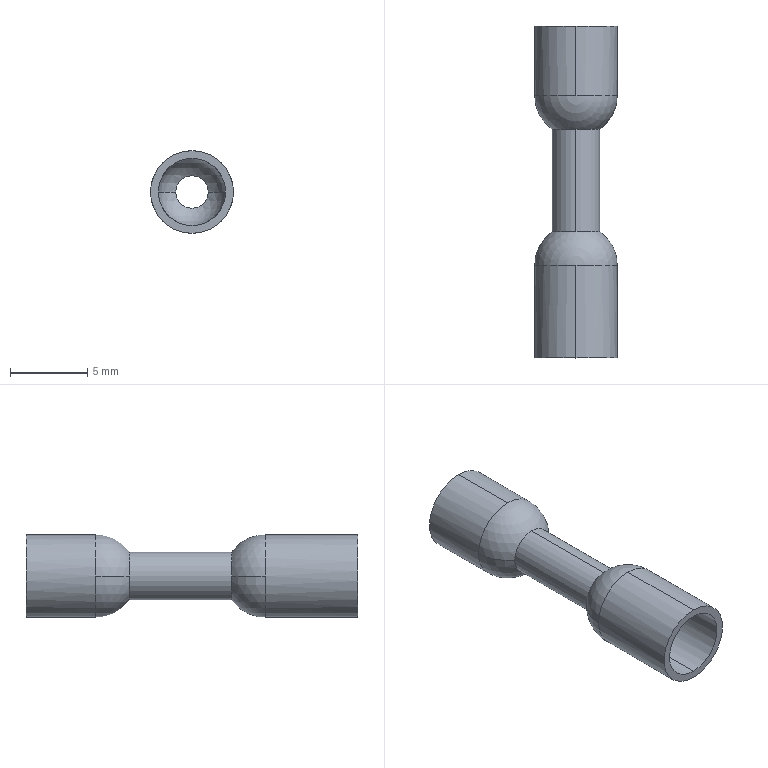Part | SolidWorks | features RevolutionThin 1 | 1 solid | 22 faces | box 5.36 x 21.494 x 5.36 mm | volume 139.623 mm3 | cylinder 12 | sphere 8 | plane 2 | commonest cylinder face diameters 4.36 x4 5.36 x4 2.1 x2 3.1 x2
STEP:
#1=CARTESIAN_POINT('',(0.,6.,2.68));
#2=VERTEX_POINT('',#1);
#3=CARTESIAN_POINT('',(2.68,6.,0.));
#4=VERTEX_POINT('',#3);
#5=CARTESIAN_POINT('',(0.,6.,0.));
#6=DIRECTION('',(0.,1.,0.));
#7=DIRECTION('',(0.,0.,1.));
#8=AXIS2_PLACEMENT_3D('',#5,#6,#7);
#9=CIRCLE('',#8,2.68);
#10=EDGE_CURVE('',#2,#4,#9,.T.);
#11=ORIENTED_EDGE('',*,*,#10,.T.);
#12=CARTESIAN_POINT('',(1.55,8.186,0.));
#13=VERTEX_POINT('',#12);
#14=CARTESIAN_POINT('',(0.,6.,0.));
#15=DIRECTION('',(0.,0.,1.));
#16=DIRECTION('',(1.,0.,0.));
#17=AXIS2_PLACEMENT_3D('',#14,#15,#16);
#18=CIRCLE('',#17,2.68);
#19=EDGE_CURVE('',#4,#13,#18,.T.);
#20=ORIENTED_EDGE('',*,*,#19,.T.);
#21=CARTESIAN_POINT('',(0.,8.186,1.55));
#22=VERTEX_POINT('',#21);
#23=CARTESIAN_POINT('',(0.,8.186,0.));
#24=DIRECTION('',(0.,1.,0.));
#25=DIRECTION('',(0.,0.,1.));
#26=AXIS2_PLACEMENT_3D('',#23,#24,#25);
#27=CIRCLE('',#26,1.55);
#28=EDGE_CURVE('',#22,#13,#27,.T.);
#29=ORIENTED_EDGE('',*,*,#28,.F.);
#30=CARTESIAN_POINT('',(-1.55,8.186,0.));
#31=VERTEX_POINT('',#30);
#32=CARTESIAN_POINT('',(0.,8.186,0.));
#33=DIRECTION('',(0.,1.,0.));
#34=DIRECTION('',(0.,0.,1.));
#35=AXIS2_PLACEMENT_3D('',#32,#33,#34);
#36=CIRCLE('',#35,1.55);
#37=EDGE_CURVE('',#31,#22,#36,.T.);
#38=ORIENTED_EDGE('',*,*,#37,.F.);
#39=CARTESIAN_POINT('',(-2.68,6.,0.));
#40=VERTEX_POINT('',#39);
#41=CARTESIAN_POINT('',(0.,6.,0.));
#42=DIRECTION('',(0.,0.,-1.));
#43=DIRECTION('',(-1.,0.,0.));
#44=AXIS2_PLACEMENT_3D('',#41,#42,#43);
#45=CIRCLE('',#44,2.68);
#46=EDGE_CURVE('',#40,#31,#45,.T.);
#47=ORIENTED_EDGE('',*,*,#46,.F.);
#48=CARTESIAN_POINT('',(0.,6.,0.));
#49=DIRECTION('',(0.,1.,0.));
#50=DIRECTION('',(0.,0.,1.));
#51=AXIS2_PLACEMENT_3D('',#48,#49,#50);
#52=CIRCLE('',#51,2.68);
#53=EDGE_CURVE('',#40,#2,#52,.T.);
#54=ORIENTED_EDGE('',*,*,#53,.T.);
#55=EDGE_LOOP('',(#11,#20,#29,#38,#47,#54));
#56=FACE_OUTER_BOUND('',#55,.T.);
#57=CARTESIAN_POINT('',(0.,6.,0.));
#58=DIRECTION('',(0.,0.,1.));
#59=DIRECTION('',(-1.,0.,0.));
#60=AXIS2_PLACEMENT_3D('',#57,#58,#59);
#61=SPHERICAL_SURFACE('',#60,2.68);
#62=ADVANCED_FACE('',(#56),#61,.T.);
#63=ORIENTED_EDGE('',*,*,#28,.T.);
#64=CARTESIAN_POINT('',(0.,8.186,-1.55));
#65=VERTEX_POINT('',#64);
#66=CARTESIAN_POINT('',(0.,8.186,0.));
#67=DIRECTION('',(0.,1.,0.));
#68=DIRECTION('',(0.,0.,1.));
#69=AXIS2_PLACEMENT_3D('',#66,#67,#68);
#70=CIRCLE('',#69,1.55);
#71=EDGE_CURVE('',#13,#65,#70,.T.);
#72=ORIENTED_EDGE('',*,*,#71,.T.);
#73=CARTESIAN_POINT('',(0.,14.808,-1.55));
#74=VERTEX_POINT('',#73);
#75=CARTESIAN_POINT('',(0.,24.172,-1.55));
#76=DIRECTION('',(0.,1.,0.));
#77=VECTOR('',#76,1000.);
#78=LINE('',#75,#77);
#79=EDGE_CURVE('',#65,#74,#78,.T.);
#80=ORIENTED_EDGE('',*,*,#79,.T.);
#81=CARTESIAN_POINT('',(1.55,14.808,0.));
#82=VERTEX_POINT('',#81);
#83=CARTESIAN_POINT('',(0.,14.808,0.));
#84=DIRECTION('',(0.,1.,0.));
#85=DIRECTION('',(0.,0.,1.));
#86=AXIS2_PLACEMENT_3D('',#83,#84,#85);
#87=CIRCLE('',#86,1.55);
#88=EDGE_CURVE('',#82,#74,#87,.T.);
#89=ORIENTED_EDGE('',*,*,#88,.F.);
#90=CARTESIAN_POINT('',(0.,14.808,1.55));
#91=VERTEX_POINT('',#90);
#92=CARTESIAN_POINT('',(0.,14.808,0.));
#93=DIRECTION('',(0.,1.,0.));
#94=DIRECTION('',(0.,0.,1.));
#95=AXIS2_PLACEMENT_3D('',#92,#93,#94);
#96=CIRCLE('',#95,1.55);
#97=EDGE_CURVE('',#91,#82,#96,.T.);
#98=ORIENTED_EDGE('',*,*,#97,.F.);
#99=CARTESIAN_POINT('',(0.,24.172,1.55));
#100=DIRECTION('',(0.,1.,0.));
#101=VECTOR('',#100,1000.);
#102=LINE('',#99,#101);
#103=EDGE_CURVE('',#22,#91,#102,.T.);
#104=ORIENTED_EDGE('',*,*,#103,.F.);
#105=EDGE_LOOP('',(#63,#72,#80,#89,#98,#104));
#106=FACE_OUTER_BOUND('',#105,.T.);
#107=CARTESIAN_POINT('',(0.,24.172,0.));
#108=DIRECTION('',(0.,1.,0.));
#109=DIRECTION('',(0.,0.,1.));
#110=AXIS2_PLACEMENT_3D('',#107,#108,#109);
#111=CYLINDRICAL_SURFACE('',#110,1.55);
#112=ADVANCED_FACE('',(#106),#111,.T.);
#113=CARTESIAN_POINT('',(-1.55,14.808,0.));
#114=VERTEX_POINT('',#113);
#115=CARTESIAN_POINT('',(0.,14.808,0.));
#116=DIRECTION('',(0.,1.,0.));
#117=DIRECTION('',(0.,0.,1.));
#118=AXIS2_PLACEMENT_3D('',#115,#116,#117);
#119=CIRCLE('',#118,1.55);
#120=EDGE_CURVE('',#114,#91,#119,.T.);
#121=ORIENTED_EDGE('',*,*,#120,.T.);
#122=ORIENTED_EDGE('',*,*,#97,.T.);
#123=CARTESIAN_POINT('',(2.68,16.994,0.));
#124=VERTEX_POINT('',#123);
#125=CARTESIAN_POINT('',(0.,16.994,0.));
#126=DIRECTION('',(0.,0.,1.));
#127=DIRECTION('',(1.,0.,0.));
#128=AXIS2_PLACEMENT_3D('',#125,#126,#127);
#129=CIRCLE('',#128,2.68);
#130=EDGE_CURVE('',#82,#124,#129,.T.);
#131=ORIENTED_EDGE('',*,*,#130,.T.);
#132=CARTESIAN_POINT('',(0.,16.994,2.68));
#133=VERTEX_POINT('',#132);
#134=CARTESIAN_POINT('',(0.,16.994,0.));
#135=DIRECTION('',(0.,1.,0.));
#136=DIRECTION('',(0.,0.,1.));
#137=AXIS2_PLACEMENT_3D('',#134,#135,#136);
#138=CIRCLE('',#137,2.68);
#139=EDGE_CURVE('',#133,#124,#138,.T.);
#140=ORIENTED_EDGE('',*,*,#139,.F.);
#141=CARTESIAN_POINT('',(-2.68,16.994,0.));
#142=VERTEX_POINT('',#141);
#143=CARTESIAN_POINT('',(0.,16.994,0.));
#144=DIRECTION('',(0.,1.,0.));
#145=DIRECTION('',(0.,0.,1.));
#146=AXIS2_PLACEMENT_3D('',#143,#144,#145);
#147=CIRCLE('',#146,2.68);
#148=EDGE_CURVE('',#142,#133,#147,.T.);
#149=ORIENTED_EDGE('',*,*,#148,.F.);
#150=CARTESIAN_POINT('',(0.,16.994,0.));
#151=DIRECTION('',(0.,0.,-1.));
#152=DIRECTION('',(-1.,0.,0.));
#153=AXIS2_PLACEMENT_3D('',#150,#151,#152);
#154=CIRCLE('',#153,2.68);
#155=EDGE_CURVE('',#114,#142,#154,.T.);
#156=ORIENTED_EDGE('',*,*,#155,.F.);
#157=EDGE_LOOP('',(#121,#122,#131,#140,#149,#156));
#158=FACE_OUTER_BOUND('',#157,.T.);
#159=CARTESIAN_POINT('',(0.,16.994,0.));
#160=DIRECTION('',(0.,0.,1.));
#161=DIRECTION('',(-1.,0.,0.));
#162=AXIS2_PLACEMENT_3D('',#159,#160,#161);
#163=SPHERICAL_SURFACE('',#162,2.68);
#164=ADVANCED_FACE('',(#158),#163,.T.);
#165=ORIENTED_EDGE('',*,*,#139,.T.);
#166=CARTESIAN_POINT('',(0.,16.994,-2.68));
#167=VERTEX_POINT('',#166);
#168=CARTESIAN_POINT('',(0.,16.994,0.));
#169=DIRECTION('',(0.,1.,0.));
#170=DIRECTION('',(0.,0.,1.));
#171=AXIS2_PLACEMENT_3D('',#168,#169,#170);
#172=CIRCLE('',#171,2.68);
#173=EDGE_CURVE('',#124,#167,#172,.T.);
#174=ORIENTED_EDGE('',*,*,#173,.T.);
#175=CARTESIAN_POINT('',(0.,21.494,-2.68));
#176=VERTEX_POINT('',#175);
#177=CARTESIAN_POINT('',(0.,24.172,-2.68));
#178=DIRECTION('',(0.,1.,0.));
#179=VECTOR('',#178,1000.);
#180=LINE('',#177,#179);
#181=EDGE_CURVE('',#167,#176,#180,.T.);
#182=ORIENTED_EDGE('',*,*,#181,.T.);
#183=CARTESIAN_POINT('',(0.,21.494,2.68));
#184=VERTEX_POINT('',#183);
#185=CARTESIAN_POINT('',(0.,21.494,0.));
#186=DIRECTION('',(0.,1.,0.));
#187=DIRECTION('',(0.,0.,1.));
#188=AXIS2_PLACEMENT_3D('',#185,#186,#187);
#189=CIRCLE('',#188,2.68);
#190=EDGE_CURVE('',#184,#176,#189,.T.);
#191=ORIENTED_EDGE('',*,*,#190,.F.);
#192=CARTESIAN_POINT('',(0.,24.172,2.68));
#193=DIRECTION('',(0.,1.,0.));
#194=VECTOR('',#193,1000.);
#195=LINE('',#192,#194);
#196=EDGE_CURVE('',#133,#184,#195,.T.);
#197=ORIENTED_EDGE('',*,*,#196,.F.);
#198=EDGE_LOOP('',(#165,#174,#182,#191,#197));
#199=FACE_OUTER_BOUND('',#198,.T.);
#200=CARTESIAN_POINT('',(0.,24.172,0.));
#201=DIRECTION('',(0.,1.,0.));
#202=DIRECTION('',(0.,0.,1.));
#203=AXIS2_PLACEMENT_3D('',#200,#201,#202);
#204=CYLINDRICAL_SURFACE('',#203,2.68);
#205=ADVANCED_FACE('',(#199),#204,.T.);
#206=CARTESIAN_POINT('',(0.,16.994,-2.18));
#207=VERTEX_POINT('',#206);
#208=CARTESIAN_POINT('',(-2.18,16.994,0.));
#209=VERTEX_POINT('',#208);
#210=CARTESIAN_POINT('',(0.,16.994,0.));
#211=DIRECTION('',(0.,1.,0.));
#212=DIRECTION('',(0.,0.,1.));
#213=AXIS2_PLACEMENT_3D('',#210,#211,#212);
#214=CIRCLE('',#213,2.18);
#215=EDGE_CURVE('',#207,#209,#214,.T.);
#216=ORIENTED_EDGE('',*,*,#215,.F.);
#217=CARTESIAN_POINT('',(0.,21.494,-2.18));
#218=VERTEX_POINT('',#217);
#219=CARTESIAN_POINT('',(0.,24.172,-2.18));
#220=DIRECTION('',(0.,1.,0.));
#221=VECTOR('',#220,1000.);
#222=LINE('',#219,#221);
#223=EDGE_CURVE('',#207,#218,#222,.T.);
#224=ORIENTED_EDGE('',*,*,#223,.T.);
#225=CARTESIAN_POINT('',(0.,21.494,2.18));
#226=VERTEX_POINT('',#225);
#227=CARTESIAN_POINT('',(0.,21.494,0.));
#228=DIRECTION('',(0.,1.,0.));
#229=DIRECTION('',(0.,0.,1.));
#230=AXIS2_PLACEMENT_3D('',#227,#228,#229);
#231=CIRCLE('',#230,2.18);
#232=EDGE_CURVE('',#218,#226,#231,.T.);
#233=ORIENTED_EDGE('',*,*,#232,.T.);
#234=CARTESIAN_POINT('',(0.,16.994,2.18));
#235=VERTEX_POINT('',#234);
#236=CARTESIAN_POINT('',(0.,24.172,2.18));
#237=DIRECTION('',(0.,1.,0.));
#238=VECTOR('',#237,1000.);
#239=LINE('',#236,#238);
#240=EDGE_CURVE('',#235,#226,#239,.T.);
#241=ORIENTED_EDGE('',*,*,#240,.F.);
#242=CARTESIAN_POINT('',(0.,16.994,0.));
#243=DIRECTION('',(0.,1.,0.));
#244=DIRECTION('',(0.,0.,1.));
#245=AXIS2_PLACEMENT_3D('',#242,#243,#244);
#246=CIRCLE('',#245,2.18);
#247=EDGE_CURVE('',#209,#235,#246,.T.);
#248=ORIENTED_EDGE('',*,*,#247,.F.);
#249=EDGE_LOOP('',(#216,#224,#233,#241,#248));
#250=FACE_OUTER_BOUND('',#249,.T.);
#251=CARTESIAN_POINT('',(0.,24.172,0.));
#252=DIRECTION('',(0.,1.,0.));
#253=DIRECTION('',(0.,0.,1.));
#254=AXIS2_PLACEMENT_3D('',#251,#252,#253);
#255=CYLINDRICAL_SURFACE('',#254,2.18);
#256=ADVANCED_FACE('',(#250),#255,.F.);
#257=CARTESIAN_POINT('',(1.05,15.083,0.));
#258=VERTEX_POINT('',#257);
#259=CARTESIAN_POINT('',(0.,15.083,-1.05));
#260=VERTEX_POINT('',#259);
#261=CARTESIAN_POINT('',(0.,15.083,0.));
#262=DIRECTION('',(0.,1.,0.));
#263=DIRECTION('',(0.,0.,1.));
#264=AXIS2_PLACEMENT_3D('',#261,#262,#263);
#265=CIRCLE('',#264,1.05);
#266=EDGE_CURVE('',#258,#260,#265,.T.);
#267=ORIENTED_EDGE('',*,*,#266,.F.);
#268=CARTESIAN_POINT('',(2.18,16.994,0.));
#269=VERTEX_POINT('',#268);
#270=CARTESIAN_POINT('',(0.,16.994,0.));
#271=DIRECTION('',(0.,0.,1.));
#272=DIRECTION('',(1.,0.,0.));
#273=AXIS2_PLACEMENT_3D('',#270,#271,#272);
#274=CIRCLE('',#273,2.18);
#275=EDGE_CURVE('',#258,#269,#274,.T.);
#276=ORIENTED_EDGE('',*,*,#275,.T.);
#277=CARTESIAN_POINT('',(0.,16.994,0.));
#278=DIRECTION('',(0.,1.,0.));
#279=DIRECTION('',(0.,0.,1.));
#280=AXIS2_PLACEMENT_3D('',#277,#278,#279);
#281=CIRCLE('',#280,2.18);
#282=EDGE_CURVE('',#269,#207,#281,.T.);
#283=ORIENTED_EDGE('',*,*,#282,.T.);
#284=ORIENTED_EDGE('',*,*,#215,.T.);
#285=CARTESIAN_POINT('',(-1.05,15.083,0.));
#286=VERTEX_POINT('',#285);
#287=CARTESIAN_POINT('',(0.,16.994,0.));
#288=DIRECTION('',(0.,0.,-1.));
#289=DIRECTION('',(-1.,0.,0.));
#290=AXIS2_PLACEMENT_3D('',#287,#288,#289);
#291=CIRCLE('',#290,2.18);
#292=EDGE_CURVE('',#286,#209,#291,.T.);
#293=ORIENTED_EDGE('',*,*,#292,.F.);
#294=CARTESIAN_POINT('',(0.,15.083,0.));
#295=DIRECTION('',(0.,1.,0.));
#296=DIRECTION('',(0.,0.,1.));
#297=AXIS2_PLACEMENT_3D('',#294,#295,#296);
#298=CIRCLE('',#297,1.05);
#299=EDGE_CURVE('',#260,#286,#298,.T.);
#300=ORIENTED_EDGE('',*,*,#299,.F.);
#301=EDGE_LOOP('',(#267,#276,#283,#284,#293,#300));
#302=FACE_OUTER_BOUND('',#301,.T.);
#303=CARTESIAN_POINT('',(0.,16.994,0.));
#304=DIRECTION('',(0.,0.,1.));
#305=DIRECTION('',(-1.,0.,0.));
#306=AXIS2_PLACEMENT_3D('',#303,#304,#305);
#307=SPHERICAL_SURFACE('',#306,2.18);
#308=ADVANCED_FACE('',(#302),#307,.F.);
#309=CARTESIAN_POINT('',(0.,7.91,-1.05));
#310=VERTEX_POINT('',#309);
#311=CARTESIAN_POINT('',(-1.05,7.91,0.));
#312=VERTEX_POINT('',#311);
#313=CARTESIAN_POINT('',(0.,7.91,0.));
#314=DIRECTION('',(0.,1.,0.));
#315=DIRECTION('',(0.,0.,1.));
#316=AXIS2_PLACEMENT_3D('',#313,#314,#315);
#317=CIRCLE('',#316,1.05);
#318=EDGE_CURVE('',#310,#312,#317,.T.);
#319=ORIENTED_EDGE('',*,*,#318,.F.);
#320=CARTESIAN_POINT('',(0.,24.172,-1.05));
#321=DIRECTION('',(0.,1.,0.));
#322=VECTOR('',#321,1000.);
#323=LINE('',#320,#322);
#324=EDGE_CURVE('',#310,#260,#323,.T.);
#325=ORIENTED_EDGE('',*,*,#324,.T.);
#326=ORIENTED_EDGE('',*,*,#299,.T.);
#327=CARTESIAN_POINT('',(0.,15.083,1.05));
#328=VERTEX_POINT('',#327);
#329=CARTESIAN_POINT('',(0.,15.083,0.));
#330=DIRECTION('',(0.,1.,0.));
#331=DIRECTION('',(0.,0.,1.));
#332=AXIS2_PLACEMENT_3D('',#329,#330,#331);
#333=CIRCLE('',#332,1.05);
#334=EDGE_CURVE('',#286,#328,#333,.T.);
#335=ORIENTED_EDGE('',*,*,#334,.T.);
#336=CARTESIAN_POINT('',(0.,7.91,1.05));
#337=VERTEX_POINT('',#336);
#338=CARTESIAN_POINT('',(0.,24.172,1.05));
#339=DIRECTION('',(0.,1.,0.));
#340=VECTOR('',#339,1000.);
#341=LINE('',#338,#340);
#342=EDGE_CURVE('',#337,#328,#341,.T.);
#343=ORIENTED_EDGE('',*,*,#342,.F.);
#344=CARTESIAN_POINT('',(0.,7.91,0.));
#345=DIRECTION('',(0.,1.,0.));
#346=DIRECTION('',(0.,0.,1.));
#347=AXIS2_PLACEMENT_3D('',#344,#345,#346);
#348=CIRCLE('',#347,1.05);
#349=EDGE_CURVE('',#312,#337,#348,.T.);
#350=ORIENTED_EDGE('',*,*,#349,.F.);
#351=EDGE_LOOP('',(#319,#325,#326,#335,#343,#350));
#352=FACE_OUTER_BOUND('',#351,.T.);
#353=CARTESIAN_POINT('',(0.,24.172,0.));
#354=DIRECTION('',(0.,1.,0.));
#355=DIRECTION('',(0.,0.,1.));
#356=AXIS2_PLACEMENT_3D('',#353,#354,#355);
#357=CYLINDRICAL_SURFACE('',#356,1.05);
#358=ADVANCED_FACE('',(#352),#357,.F.);
#359=CARTESIAN_POINT('',(2.18,6.,0.));
#360=VERTEX_POINT('',#359);
#361=CARTESIAN_POINT('',(0.,6.,-2.18));
#362=VERTEX_POINT('',#361);
#363=CARTESIAN_POINT('',(0.,6.,0.));
#364=DIRECTION('',(0.,1.,0.));
#365=DIRECTION('',(0.,0.,1.));
#366=AXIS2_PLACEMENT_3D('',#363,#364,#365);
#367=CIRCLE('',#366,2.18);
#368=EDGE_CURVE('',#360,#362,#367,.T.);
#369=ORIENTED_EDGE('',*,*,#368,.F.);
#370=CARTESIAN_POINT('',(1.05,7.91,0.));
#371=VERTEX_POINT('',#370);
#372=CARTESIAN_POINT('',(0.,6.,0.));
#373=DIRECTION('',(0.,0.,1.));
#374=DIRECTION('',(1.,0.,0.));
#375=AXIS2_PLACEMENT_3D('',#372,#373,#374);
#376=CIRCLE('',#375,2.18);
#377=EDGE_CURVE('',#360,#371,#376,.T.);
#378=ORIENTED_EDGE('',*,*,#377,.T.);
#379=CARTESIAN_POINT('',(0.,7.91,0.));
#380=DIRECTION('',(0.,1.,0.));
#381=DIRECTION('',(0.,0.,1.));
#382=AXIS2_PLACEMENT_3D('',#379,#380,#381);
#383=CIRCLE('',#382,1.05);
#384=EDGE_CURVE('',#371,#310,#383,.T.);
#385=ORIENTED_EDGE('',*,*,#384,.T.);
#386=ORIENTED_EDGE('',*,*,#318,.T.);
#387=CARTESIAN_POINT('',(-2.18,6.,0.));
#388=VERTEX_POINT('',#387);
#389=CARTESIAN_POINT('',(0.,6.,0.));
#390=DIRECTION('',(0.,0.,-1.));
#391=DIRECTION('',(-1.,0.,0.));
#392=AXIS2_PLACEMENT_3D('',#389,#390,#391);
#393=CIRCLE('',#392,2.18);
#394=EDGE_CURVE('',#388,#312,#393,.T.);
#395=ORIENTED_EDGE('',*,*,#394,.F.);
#396=CARTESIAN_POINT('',(0.,6.,0.));
#397=DIRECTION('',(0.,1.,0.));
#398=DIRECTION('',(0.,0.,1.));
#399=AXIS2_PLACEMENT_3D('',#396,#397,#398);
#400=CIRCLE('',#399,2.18);
#401=EDGE_CURVE('',#362,#388,#400,.T.);
#402=ORIENTED_EDGE('',*,*,#401,.F.);
#403=EDGE_LOOP('',(#369,#378,#385,#386,#395,#402));
#404=FACE_OUTER_BOUND('',#403,.T.);
#405=CARTESIAN_POINT('',(0.,6.,0.));
#406=DIRECTION('',(0.,0.,1.));
#407=DIRECTION('',(-1.,0.,0.));
#408=AXIS2_PLACEMENT_3D('',#405,#406,#407);
#409=SPHERICAL_SURFACE('',#408,2.18);
#410=ADVANCED_FACE('',(#404),#409,.F.);
#411=CARTESIAN_POINT('',(0.,0.,-2.18));
#412=VERTEX_POINT('',#411);
#413=CARTESIAN_POINT('',(0.,0.,2.18));
#414=VERTEX_POINT('',#413);
#415=CARTESIAN_POINT('',(0.,0.,0.));
#416=DIRECTION('',(0.,1.,0.));
#417=DIRECTION('',(0.,0.,1.));
#418=AXIS2_PLACEMENT_3D('',#415,#416,#417);
#419=CIRCLE('',#418,2.18);
#420=EDGE_CURVE('',#412,#414,#419,.T.);
#421=ORIENTED_EDGE('',*,*,#420,.F.);
#422=CARTESIAN_POINT('',(0.,24.172,-2.18));
#423=DIRECTION('',(0.,1.,0.));
#424=VECTOR('',#423,1000.);
#425=LINE('',#422,#424);
#426=EDGE_CURVE('',#412,#362,#425,.T.);
#427=ORIENTED_EDGE('',*,*,#426,.T.);
#428=ORIENTED_EDGE('',*,*,#401,.T.);
#429=CARTESIAN_POINT('',(0.,6.,2.18));
#430=VERTEX_POINT('',#429);
#431=CARTESIAN_POINT('',(0.,6.,0.));
#432=DIRECTION('',(0.,1.,0.));
#433=DIRECTION('',(0.,0.,1.));
#434=AXIS2_PLACEMENT_3D('',#431,#432,#433);
#435=CIRCLE('',#434,2.18);
#436=EDGE_CURVE('',#388,#430,#435,.T.);
#437=ORIENTED_EDGE('',*,*,#436,.T.);
#438=CARTESIAN_POINT('',(0.,24.172,2.18));
#439=DIRECTION('',(0.,1.,0.));
#440=VECTOR('',#439,1000.);
#441=LINE('',#438,#440);
#442=EDGE_CURVE('',#414,#430,#441,.T.);
#443=ORIENTED_EDGE('',*,*,#442,.F.);
#444=EDGE_LOOP('',(#421,#427,#428,#437,#443));
#445=FACE_OUTER_BOUND('',#444,.T.);
#446=CARTESIAN_POINT('',(0.,24.172,0.));
#447=DIRECTION('',(0.,1.,0.));
#448=DIRECTION('',(0.,0.,1.));
#449=AXIS2_PLACEMENT_3D('',#446,#447,#448);
#450=CYLINDRICAL_SURFACE('',#449,2.18);
#451=ADVANCED_FACE('',(#445),#450,.F.);
#452=CARTESIAN_POINT('',(0.,0.,2.68));
#453=VERTEX_POINT('',#452);
#454=CARTESIAN_POINT('',(0.,0.,-2.68));
#455=VERTEX_POINT('',#454);
#456=CARTESIAN_POINT('',(0.,0.,0.));
#457=DIRECTION('',(0.,1.,0.));
#458=DIRECTION('',(0.,0.,1.));
#459=AXIS2_PLACEMENT_3D('',#456,#457,#458);
#460=CIRCLE('',#459,2.68);
#461=EDGE_CURVE('',#453,#455,#460,.T.);
#462=ORIENTED_EDGE('',*,*,#461,.T.);
#463=CARTESIAN_POINT('',(0.,6.,-2.68));
#464=VERTEX_POINT('',#463);
#465=CARTESIAN_POINT('',(0.,24.172,-2.68));
#466=DIRECTION('',(0.,1.,0.));
#467=VECTOR('',#466,1000.);
#468=LINE('',#465,#467);
#469=EDGE_CURVE('',#455,#464,#468,.T.);
#470=ORIENTED_EDGE('',*,*,#469,.T.);
#471=CARTESIAN_POINT('',(0.,6.,0.));
#472=DIRECTION('',(0.,1.,0.));
#473=DIRECTION('',(0.,0.,1.));
#474=AXIS2_PLACEMENT_3D('',#471,#472,#473);
#475=CIRCLE('',#474,2.68);
#476=EDGE_CURVE('',#4,#464,#475,.T.);
#477=ORIENTED_EDGE('',*,*,#476,.F.);
#478=ORIENTED_EDGE('',*,*,#10,.F.);
#479=CARTESIAN_POINT('',(0.,24.172,2.68));
#480=DIRECTION('',(0.,1.,0.));
#481=VECTOR('',#480,1000.);
#482=LINE('',#479,#481);
#483=EDGE_CURVE('',#453,#2,#482,.T.);
#484=ORIENTED_EDGE('',*,*,#483,.F.);
#485=EDGE_LOOP('',(#462,#470,#477,#478,#484));
#486=FACE_OUTER_BOUND('',#485,.T.);
#487=CARTESIAN_POINT('',(0.,24.172,0.));
#488=DIRECTION('',(0.,1.,0.));
#489=DIRECTION('',(0.,0.,1.));
#490=AXIS2_PLACEMENT_3D('',#487,#488,#489);
#491=CYLINDRICAL_SURFACE('',#490,2.68);
#492=ADVANCED_FACE('',(#486),#491,.T.);
#493=ORIENTED_EDGE('',*,*,#469,.F.);
#494=CARTESIAN_POINT('',(0.,0.,0.));
#495=DIRECTION('',(0.,1.,0.));
#496=DIRECTION('',(0.,0.,1.));
#497=AXIS2_PLACEMENT_3D('',#494,#495,#496);
#498=CIRCLE('',#497,2.68);
#499=EDGE_CURVE('',#455,#453,#498,.T.);
#500=ORIENTED_EDGE('',*,*,#499,.T.);
#501=ORIENTED_EDGE('',*,*,#483,.T.);
#502=ORIENTED_EDGE('',*,*,#53,.F.);
#503=CARTESIAN_POINT('',(0.,6.,0.));
#504=DIRECTION('',(0.,1.,0.));
#505=DIRECTION('',(0.,0.,1.));
#506=AXIS2_PLACEMENT_3D('',#503,#504,#505);
#507=CIRCLE('',#506,2.68);
#508=EDGE_CURVE('',#464,#40,#507,.T.);
#509=ORIENTED_EDGE('',*,*,#508,.F.);
#510=EDGE_LOOP('',(#493,#500,#501,#502,#509));
#511=FACE_OUTER_BOUND('',#510,.T.);
#512=CARTESIAN_POINT('',(0.,24.172,0.));
#513=DIRECTION('',(0.,1.,0.));
#514=DIRECTION('',(0.,0.,1.));
#515=AXIS2_PLACEMENT_3D('',#512,#513,#514);
#516=CYLINDRICAL_SURFACE('',#515,2.68);
#517=ADVANCED_FACE('',(#511),#516,.T.);
#518=ORIENTED_EDGE('',*,*,#461,.F.);
#519=ORIENTED_EDGE('',*,*,#499,.F.);
#520=EDGE_LOOP('',(#518,#519));
#521=FACE_OUTER_BOUND('',#520,.T.);
#522=CARTESIAN_POINT('',(0.,0.,0.));
#523=DIRECTION('',(0.,1.,0.));
#524=DIRECTION('',(0.,0.,1.));
#525=AXIS2_PLACEMENT_3D('',#522,#523,#524);
#526=CIRCLE('',#525,2.18);
#527=EDGE_CURVE('',#414,#412,#526,.T.);
#528=ORIENTED_EDGE('',*,*,#527,.T.);
#529=ORIENTED_EDGE('',*,*,#420,.T.);
#530=EDGE_LOOP('',(#528,#529));
#531=FACE_BOUND('',#530,.T.);
#532=CARTESIAN_POINT('',(-2.18,0.,0.));
#533=DIRECTION('',(0.,1.,0.));
#534=DIRECTION('',(0.,0.,1.));
#535=AXIS2_PLACEMENT_3D('',#532,#533,#534);
#536=PLANE('',#535);
#537=ADVANCED_FACE('',(#521,#531),#536,.F.);
#538=ORIENTED_EDGE('',*,*,#426,.F.);
#539=ORIENTED_EDGE('',*,*,#527,.F.);
#540=ORIENTED_EDGE('',*,*,#442,.T.);
#541=CARTESIAN_POINT('',(0.,6.,0.));
#542=DIRECTION('',(0.,1.,0.));
#543=DIRECTION('',(0.,0.,1.));
#544=AXIS2_PLACEMENT_3D('',#541,#542,#543);
#545=CIRCLE('',#544,2.18);
#546=EDGE_CURVE('',#430,#360,#545,.T.);
#547=ORIENTED_EDGE('',*,*,#546,.T.);
#548=ORIENTED_EDGE('',*,*,#368,.T.);
#549=EDGE_LOOP('',(#538,#539,#540,#547,#548));
#550=FACE_OUTER_BOUND('',#549,.T.);
#551=CARTESIAN_POINT('',(0.,24.172,0.));
#552=DIRECTION('',(0.,1.,0.));
#553=DIRECTION('',(0.,0.,1.));
#554=AXIS2_PLACEMENT_3D('',#551,#552,#553);
#555=CYLINDRICAL_SURFACE('',#554,2.18);
#556=ADVANCED_FACE('',(#550),#555,.F.);
#557=ORIENTED_EDGE('',*,*,#377,.F.);
#558=ORIENTED_EDGE('',*,*,#546,.F.);
#559=ORIENTED_EDGE('',*,*,#436,.F.);
#560=ORIENTED_EDGE('',*,*,#394,.T.);
#561=ORIENTED_EDGE('',*,*,#349,.T.);
#562=CARTESIAN_POINT('',(0.,7.91,0.));
#563=DIRECTION('',(0.,1.,0.));
#564=DIRECTION('',(0.,0.,1.));
#565=AXIS2_PLACEMENT_3D('',#562,#563,#564);
#566=CIRCLE('',#565,1.05);
#567=EDGE_CURVE('',#337,#371,#566,.T.);
#568=ORIENTED_EDGE('',*,*,#567,.T.);
#569=EDGE_LOOP('',(#557,#558,#559,#560,#561,#568));
#570=FACE_OUTER_BOUND('',#569,.T.);
#571=CARTESIAN_POINT('',(0.,6.,0.));
#572=DIRECTION('',(0.,0.,1.));
#573=DIRECTION('',(-1.,0.,0.));
#574=AXIS2_PLACEMENT_3D('',#571,#572,#573);
#575=SPHERICAL_SURFACE('',#574,2.18);
#576=ADVANCED_FACE('',(#570),#575,.F.);
#577=ORIENTED_EDGE('',*,*,#324,.F.);
#578=ORIENTED_EDGE('',*,*,#384,.F.);
#579=ORIENTED_EDGE('',*,*,#567,.F.);
#580=ORIENTED_EDGE('',*,*,#342,.T.);
#581=CARTESIAN_POINT('',(0.,15.083,0.));
#582=DIRECTION('',(0.,1.,0.));
#583=DIRECTION('',(0.,0.,1.));
#584=AXIS2_PLACEMENT_3D('',#581,#582,#583);
#585=CIRCLE('',#584,1.05);
#586=EDGE_CURVE('',#328,#258,#585,.T.);
#587=ORIENTED_EDGE('',*,*,#586,.T.);
#588=ORIENTED_EDGE('',*,*,#266,.T.);
#589=EDGE_LOOP('',(#577,#578,#579,#580,#587,#588));
#590=FACE_OUTER_BOUND('',#589,.T.);
#591=CARTESIAN_POINT('',(0.,24.172,0.));
#592=DIRECTION('',(0.,1.,0.));
#593=DIRECTION('',(0.,0.,1.));
#594=AXIS2_PLACEMENT_3D('',#591,#592,#593);
#595=CYLINDRICAL_SURFACE('',#594,1.05);
#596=ADVANCED_FACE('',(#590),#595,.F.);
#597=ORIENTED_EDGE('',*,*,#275,.F.);
#598=ORIENTED_EDGE('',*,*,#586,.F.);
#599=ORIENTED_EDGE('',*,*,#334,.F.);
#600=ORIENTED_EDGE('',*,*,#292,.T.);
#601=ORIENTED_EDGE('',*,*,#247,.T.);
#602=CARTESIAN_POINT('',(0.,16.994,0.));
#603=DIRECTION('',(0.,1.,0.));
#604=DIRECTION('',(0.,0.,1.));
#605=AXIS2_PLACEMENT_3D('',#602,#603,#604);
#606=CIRCLE('',#605,2.18);
#607=EDGE_CURVE('',#235,#269,#606,.T.);
#608=ORIENTED_EDGE('',*,*,#607,.T.);
#609=EDGE_LOOP('',(#597,#598,#599,#600,#601,#608));
#610=FACE_OUTER_BOUND('',#609,.T.);
#611=CARTESIAN_POINT('',(0.,16.994,0.));
#612=DIRECTION('',(0.,0.,1.));
#613=DIRECTION('',(-1.,0.,0.));
#614=AXIS2_PLACEMENT_3D('',#611,#612,#613);
#615=SPHERICAL_SURFACE('',#614,2.18);
#616=ADVANCED_FACE('',(#610),#615,.F.);
#617=ORIENTED_EDGE('',*,*,#223,.F.);
#618=ORIENTED_EDGE('',*,*,#282,.F.);
#619=ORIENTED_EDGE('',*,*,#607,.F.);
#620=ORIENTED_EDGE('',*,*,#240,.T.);
#621=CARTESIAN_POINT('',(0.,21.494,0.));
#622=DIRECTION('',(0.,1.,0.));
#623=DIRECTION('',(0.,0.,1.));
#624=AXIS2_PLACEMENT_3D('',#621,#622,#623);
#625=CIRCLE('',#624,2.18);
#626=EDGE_CURVE('',#226,#218,#625,.T.);
#627=ORIENTED_EDGE('',*,*,#626,.T.);
#628=EDGE_LOOP('',(#617,#618,#619,#620,#627));
#629=FACE_OUTER_BOUND('',#628,.T.);
#630=CARTESIAN_POINT('',(0.,24.172,0.));
#631=DIRECTION('',(0.,1.,0.));
#632=DIRECTION('',(0.,0.,1.));
#633=AXIS2_PLACEMENT_3D('',#630,#631,#632);
#634=CYLINDRICAL_SURFACE('',#633,2.18);
#635=ADVANCED_FACE('',(#629),#634,.F.);
#636=ORIENTED_EDGE('',*,*,#626,.F.);
#637=ORIENTED_EDGE('',*,*,#232,.F.);
#638=EDGE_LOOP('',(#636,#637));
#639=FACE_BOUND('',#638,.T.);
#640=ORIENTED_EDGE('',*,*,#190,.T.);
#641=CARTESIAN_POINT('',(0.,21.494,0.));
#642=DIRECTION('',(0.,1.,0.));
#643=DIRECTION('',(0.,0.,1.));
#644=AXIS2_PLACEMENT_3D('',#641,#642,#643);
#645=CIRCLE('',#644,2.68);
#646=EDGE_CURVE('',#176,#184,#645,.T.);
#647=ORIENTED_EDGE('',*,*,#646,.T.);
#648=EDGE_LOOP('',(#640,#647));
#649=FACE_OUTER_BOUND('',#648,.T.);
#650=CARTESIAN_POINT('',(-2.68,21.494,0.));
#651=DIRECTION('',(0.,-1.,0.));
#652=DIRECTION('',(0.,0.,-1.));
#653=AXIS2_PLACEMENT_3D('',#650,#651,#652);
#654=PLANE('',#653);
#655=ADVANCED_FACE('',(#639,#649),#654,.F.);
#656=ORIENTED_EDGE('',*,*,#181,.F.);
#657=CARTESIAN_POINT('',(0.,16.994,0.));
#658=DIRECTION('',(0.,1.,0.));
#659=DIRECTION('',(0.,0.,1.));
#660=AXIS2_PLACEMENT_3D('',#657,#658,#659);
#661=CIRCLE('',#660,2.68);
#662=EDGE_CURVE('',#167,#142,#661,.T.);
#663=ORIENTED_EDGE('',*,*,#662,.T.);
#664=ORIENTED_EDGE('',*,*,#148,.T.);
#665=ORIENTED_EDGE('',*,*,#196,.T.);
#666=ORIENTED_EDGE('',*,*,#646,.F.);
#667=EDGE_LOOP('',(#656,#663,#664,#665,#666));
#668=FACE_OUTER_BOUND('',#667,.T.);
#669=CARTESIAN_POINT('',(0.,24.172,0.));
#670=DIRECTION('',(0.,1.,0.));
#671=DIRECTION('',(0.,0.,1.));
#672=AXIS2_PLACEMENT_3D('',#669,#670,#671);
#673=CYLINDRICAL_SURFACE('',#672,2.68);
#674=ADVANCED_FACE('',(#668),#673,.T.);
#675=ORIENTED_EDGE('',*,*,#130,.F.);
#676=ORIENTED_EDGE('',*,*,#88,.T.);
#677=CARTESIAN_POINT('',(0.,14.808,0.));
#678=DIRECTION('',(0.,1.,0.));
#679=DIRECTION('',(0.,0.,1.));
#680=AXIS2_PLACEMENT_3D('',#677,#678,#679);
#681=CIRCLE('',#680,1.55);
#682=EDGE_CURVE('',#74,#114,#681,.T.);
#683=ORIENTED_EDGE('',*,*,#682,.T.);
#684=ORIENTED_EDGE('',*,*,#155,.T.);
#685=ORIENTED_EDGE('',*,*,#662,.F.);
#686=ORIENTED_EDGE('',*,*,#173,.F.);
#687=EDGE_LOOP('',(#675,#676,#683,#684,#685,#686));
#688=FACE_OUTER_BOUND('',#687,.T.);
#689=CARTESIAN_POINT('',(0.,16.994,0.));
#690=DIRECTION('',(0.,0.,1.));
#691=DIRECTION('',(-1.,0.,0.));
#692=AXIS2_PLACEMENT_3D('',#689,#690,#691);
#693=SPHERICAL_SURFACE('',#692,2.68);
#694=ADVANCED_FACE('',(#688),#693,.T.);
#695=ORIENTED_EDGE('',*,*,#79,.F.);
#696=CARTESIAN_POINT('',(0.,8.186,0.));
#697=DIRECTION('',(0.,1.,0.));
#698=DIRECTION('',(0.,0.,1.));
#699=AXIS2_PLACEMENT_3D('',#696,#697,#698);
#700=CIRCLE('',#699,1.55);
#701=EDGE_CURVE('',#65,#31,#700,.T.);
#702=ORIENTED_EDGE('',*,*,#701,.T.);
#703=ORIENTED_EDGE('',*,*,#37,.T.);
#704=ORIENTED_EDGE('',*,*,#103,.T.);
#705=ORIENTED_EDGE('',*,*,#120,.F.);
#706=ORIENTED_EDGE('',*,*,#682,.F.);
#707=EDGE_LOOP('',(#695,#702,#703,#704,#705,#706));
#708=FACE_OUTER_BOUND('',#707,.T.);
#709=CARTESIAN_POINT('',(0.,24.172,0.));
#710=DIRECTION('',(0.,1.,0.));
#711=DIRECTION('',(0.,0.,1.));
#712=AXIS2_PLACEMENT_3D('',#709,#710,#711);
#713=CYLINDRICAL_SURFACE('',#712,1.55);
#714=ADVANCED_FACE('',(#708),#713,.T.);
#715=ORIENTED_EDGE('',*,*,#19,.F.);
#716=ORIENTED_EDGE('',*,*,#476,.T.);
#717=ORIENTED_EDGE('',*,*,#508,.T.);
#718=ORIENTED_EDGE('',*,*,#46,.T.);
#719=ORIENTED_EDGE('',*,*,#701,.F.);
#720=ORIENTED_EDGE('',*,*,#71,.F.);
#721=EDGE_LOOP('',(#715,#716,#717,#718,#719,#720));
#722=FACE_OUTER_BOUND('',#721,.T.);
#723=CARTESIAN_POINT('',(0.,6.,0.));
#724=DIRECTION('',(0.,0.,1.));
#725=DIRECTION('',(-1.,0.,0.));
#726=AXIS2_PLACEMENT_3D('',#723,#724,#725);
#727=SPHERICAL_SURFACE('',#726,2.68);
#728=ADVANCED_FACE('',(#722),#727,.T.);
#729=CLOSED_SHELL('',(#62,#112,#164,#205,#256,#308,#358,#410,#451,#492,#517,#537,#556,#576,#596,#616,#635,#655,#674,#694,#714,#728));
#730=MANIFOLD_SOLID_BREP('',#729);
#731=CARTESIAN_POINT('',(0.,0.,0.));
#732=DIRECTION('',(0.,0.,1.));
#733=DIRECTION('',(1.,0.,0.));
#734=AXIS2_PLACEMENT_3D('',#731,#732,#733);
#735=(LENGTH_UNIT()NAMED_UNIT(*)SI_UNIT(.MILLI.,.METRE.));
#736=UNCERTAINTY_MEASURE_WITH_UNIT(LENGTH_MEASURE(0.00001),#735,'','');
#737=(NAMED_UNIT(*)PLANE_ANGLE_UNIT()SI_UNIT($,.RADIAN.));
#738=(NAMED_UNIT(*)SI_UNIT($,.STERADIAN.)SOLID_ANGLE_UNIT());
#739=(GEOMETRIC_REPRESENTATION_CONTEXT(3)GLOBAL_UNCERTAINTY_ASSIGNED_CONTEXT((#736))GLOBAL_UNIT_ASSIGNED_CONTEXT((#735,#737,#738))REPRESENTATION_CONTEXT('',''));
#740=ADVANCED_BREP_SHAPE_REPRESENTATION('',(#730,#734),#739);